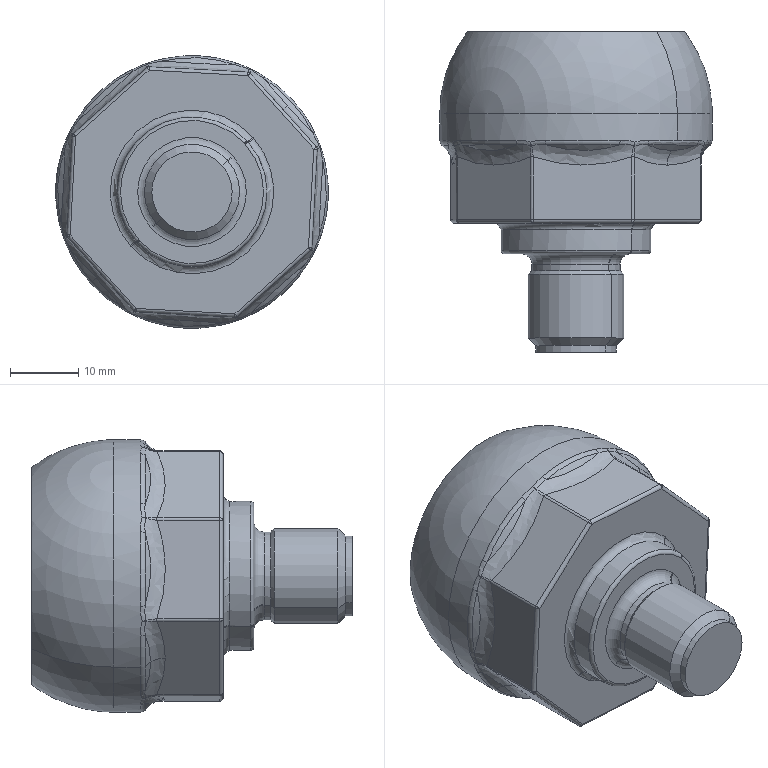Part | SolidWorks | features BaseBody 1 | 1 solid | 148 faces | box 40 x 47.036 x 40 mm | volume 19515 mm3 | spline 42 | torus 34 | cylinder 28 | cone 19 | sphere 14 | plane 11 | commonest cylinder face diameters 1 x16 11.8 x2 12.97 x2 14 x2 22 x2 30.55 x2